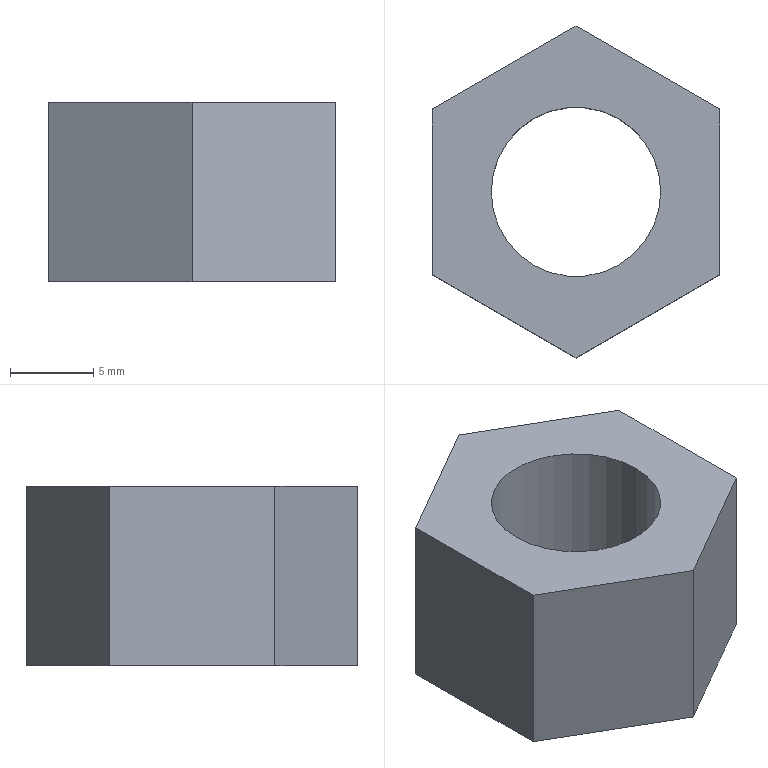Part | SolidWorks | features Extrusion 1, HoleWzd 1, RefAxis 1 | 1 solid | 10 faces | box 17.3 x 19.976 x 10.8 mm | volume 1917 mm3 | plane 8 | cylinder 2 | commonest cylinder face diameters 10.2 x2
STEP:
#1=CARTESIAN_POINT('',(-5.1,0.,-5.4));
#2=VERTEX_POINT('',#1);
#3=CARTESIAN_POINT('',(5.1,0.,-5.4));
#4=VERTEX_POINT('',#3);
#5=CARTESIAN_POINT('',(0.,0.,-5.4));
#6=DIRECTION('',(0.,0.,1.));
#7=DIRECTION('',(1.,0.,0.));
#8=AXIS2_PLACEMENT_3D('',#5,#6,#7);
#9=CIRCLE('',#8,5.1);
#10=EDGE_CURVE('',#2,#4,#9,.T.);
#11=ORIENTED_EDGE('',*,*,#10,.F.);
#12=CARTESIAN_POINT('',(-5.1,0.,5.4));
#13=VERTEX_POINT('',#12);
#14=CARTESIAN_POINT('',(-5.1,0.,5.4));
#15=DIRECTION('',(0.,0.,1.));
#16=VECTOR('',#15,1000.);
#17=LINE('',#14,#16);
#18=EDGE_CURVE('',#2,#13,#17,.T.);
#19=ORIENTED_EDGE('',*,*,#18,.T.);
#20=CARTESIAN_POINT('',(5.1,0.,5.4));
#21=VERTEX_POINT('',#20);
#22=CARTESIAN_POINT('',(0.,0.,5.4));
#23=DIRECTION('',(0.,0.,1.));
#24=DIRECTION('',(1.,0.,0.));
#25=AXIS2_PLACEMENT_3D('',#22,#23,#24);
#26=CIRCLE('',#25,5.1);
#27=EDGE_CURVE('',#13,#21,#26,.T.);
#28=ORIENTED_EDGE('',*,*,#27,.T.);
#29=CARTESIAN_POINT('',(5.1,0.,5.4));
#30=DIRECTION('',(0.,0.,1.));
#31=VECTOR('',#30,1000.);
#32=LINE('',#29,#31);
#33=EDGE_CURVE('',#4,#21,#32,.T.);
#34=ORIENTED_EDGE('',*,*,#33,.F.);
#35=EDGE_LOOP('',(#11,#19,#28,#34));
#36=FACE_OUTER_BOUND('',#35,.T.);
#37=CARTESIAN_POINT('',(0.,0.,5.4));
#38=DIRECTION('',(0.,0.,1.));
#39=DIRECTION('',(1.,0.,0.));
#40=AXIS2_PLACEMENT_3D('',#37,#38,#39);
#41=CYLINDRICAL_SURFACE('',#40,5.1);
#42=ADVANCED_FACE('',(#36),#41,.F.);
#43=CARTESIAN_POINT('',(0.,-9.988,-5.4));
#44=VERTEX_POINT('',#43);
#45=CARTESIAN_POINT('',(8.65,-4.994,-5.4));
#46=VERTEX_POINT('',#45);
#47=CARTESIAN_POINT('',(0.,-9.988,-5.4));
#48=DIRECTION('',(0.866,0.5,0.));
#49=VECTOR('',#48,1000.);
#50=LINE('',#47,#49);
#51=EDGE_CURVE('',#44,#46,#50,.T.);
#52=ORIENTED_EDGE('',*,*,#51,.T.);
#53=CARTESIAN_POINT('',(8.65,-4.994,5.4));
#54=VERTEX_POINT('',#53);
#55=CARTESIAN_POINT('',(8.65,-4.994,5.4));
#56=DIRECTION('',(0.,0.,-1.));
#57=VECTOR('',#56,1000.);
#58=LINE('',#55,#57);
#59=EDGE_CURVE('',#54,#46,#58,.T.);
#60=ORIENTED_EDGE('',*,*,#59,.F.);
#61=CARTESIAN_POINT('',(0.,-9.988,5.4));
#62=VERTEX_POINT('',#61);
#63=CARTESIAN_POINT('',(0.,-9.988,5.4));
#64=DIRECTION('',(0.866,0.5,0.));
#65=VECTOR('',#64,1000.);
#66=LINE('',#63,#65);
#67=EDGE_CURVE('',#62,#54,#66,.T.);
#68=ORIENTED_EDGE('',*,*,#67,.F.);
#69=CARTESIAN_POINT('',(0.,-9.988,5.4));
#70=DIRECTION('',(0.,0.,-1.));
#71=VECTOR('',#70,1000.);
#72=LINE('',#69,#71);
#73=EDGE_CURVE('',#62,#44,#72,.T.);
#74=ORIENTED_EDGE('',*,*,#73,.T.);
#75=EDGE_LOOP('',(#52,#60,#68,#74));
#76=FACE_OUTER_BOUND('',#75,.T.);
#77=CARTESIAN_POINT('',(0.,-9.988,5.4));
#78=DIRECTION('',(-0.5,0.866,0.));
#79=DIRECTION('',(-0.866,-0.5,0.));
#80=AXIS2_PLACEMENT_3D('',#77,#78,#79);
#81=PLANE('',#80);
#82=ADVANCED_FACE('',(#76),#81,.F.);
#83=CARTESIAN_POINT('',(8.65,4.994,-5.4));
#84=VERTEX_POINT('',#83);
#85=CARTESIAN_POINT('',(8.65,-4.994,-5.4));
#86=DIRECTION('',(0.,1.,0.));
#87=VECTOR('',#86,1000.);
#88=LINE('',#85,#87);
#89=EDGE_CURVE('',#46,#84,#88,.T.);
#90=ORIENTED_EDGE('',*,*,#89,.T.);
#91=CARTESIAN_POINT('',(8.65,4.994,5.4));
#92=VERTEX_POINT('',#91);
#93=CARTESIAN_POINT('',(8.65,4.994,5.4));
#94=DIRECTION('',(0.,0.,-1.));
#95=VECTOR('',#94,1000.);
#96=LINE('',#93,#95);
#97=EDGE_CURVE('',#92,#84,#96,.T.);
#98=ORIENTED_EDGE('',*,*,#97,.F.);
#99=CARTESIAN_POINT('',(8.65,-4.994,5.4));
#100=DIRECTION('',(0.,1.,0.));
#101=VECTOR('',#100,1000.);
#102=LINE('',#99,#101);
#103=EDGE_CURVE('',#54,#92,#102,.T.);
#104=ORIENTED_EDGE('',*,*,#103,.F.);
#105=ORIENTED_EDGE('',*,*,#59,.T.);
#106=EDGE_LOOP('',(#90,#98,#104,#105));
#107=FACE_OUTER_BOUND('',#106,.T.);
#108=CARTESIAN_POINT('',(8.65,-4.994,5.4));
#109=DIRECTION('',(-1.,0.,0.));
#110=DIRECTION('',(0.,0.,1.));
#111=AXIS2_PLACEMENT_3D('',#108,#109,#110);
#112=PLANE('',#111);
#113=ADVANCED_FACE('',(#107),#112,.F.);
#114=CARTESIAN_POINT('',(0.,9.988,-5.4));
#115=VERTEX_POINT('',#114);
#116=CARTESIAN_POINT('',(8.65,4.994,-5.4));
#117=DIRECTION('',(-0.866,0.5,0.));
#118=VECTOR('',#117,1000.);
#119=LINE('',#116,#118);
#120=EDGE_CURVE('',#84,#115,#119,.T.);
#121=ORIENTED_EDGE('',*,*,#120,.T.);
#122=CARTESIAN_POINT('',(0.,9.988,5.4));
#123=VERTEX_POINT('',#122);
#124=CARTESIAN_POINT('',(0.,9.988,5.4));
#125=DIRECTION('',(0.,0.,-1.));
#126=VECTOR('',#125,1000.);
#127=LINE('',#124,#126);
#128=EDGE_CURVE('',#123,#115,#127,.T.);
#129=ORIENTED_EDGE('',*,*,#128,.F.);
#130=CARTESIAN_POINT('',(8.65,4.994,5.4));
#131=DIRECTION('',(-0.866,0.5,0.));
#132=VECTOR('',#131,1000.);
#133=LINE('',#130,#132);
#134=EDGE_CURVE('',#92,#123,#133,.T.);
#135=ORIENTED_EDGE('',*,*,#134,.F.);
#136=ORIENTED_EDGE('',*,*,#97,.T.);
#137=EDGE_LOOP('',(#121,#129,#135,#136));
#138=FACE_OUTER_BOUND('',#137,.T.);
#139=CARTESIAN_POINT('',(8.65,4.994,5.4));
#140=DIRECTION('',(-0.5,-0.866,0.));
#141=DIRECTION('',(0.866,-0.5,0.));
#142=AXIS2_PLACEMENT_3D('',#139,#140,#141);
#143=PLANE('',#142);
#144=ADVANCED_FACE('',(#138),#143,.F.);
#145=CARTESIAN_POINT('',(-8.65,4.994,-5.4));
#146=VERTEX_POINT('',#145);
#147=CARTESIAN_POINT('',(0.,9.988,-5.4));
#148=DIRECTION('',(-0.866,-0.5,0.));
#149=VECTOR('',#148,1000.);
#150=LINE('',#147,#149);
#151=EDGE_CURVE('',#115,#146,#150,.T.);
#152=ORIENTED_EDGE('',*,*,#151,.T.);
#153=CARTESIAN_POINT('',(-8.65,4.994,5.4));
#154=VERTEX_POINT('',#153);
#155=CARTESIAN_POINT('',(-8.65,4.994,5.4));
#156=DIRECTION('',(0.,0.,-1.));
#157=VECTOR('',#156,1000.);
#158=LINE('',#155,#157);
#159=EDGE_CURVE('',#154,#146,#158,.T.);
#160=ORIENTED_EDGE('',*,*,#159,.F.);
#161=CARTESIAN_POINT('',(0.,9.988,5.4));
#162=DIRECTION('',(-0.866,-0.5,0.));
#163=VECTOR('',#162,1000.);
#164=LINE('',#161,#163);
#165=EDGE_CURVE('',#123,#154,#164,.T.);
#166=ORIENTED_EDGE('',*,*,#165,.F.);
#167=ORIENTED_EDGE('',*,*,#128,.T.);
#168=EDGE_LOOP('',(#152,#160,#166,#167));
#169=FACE_OUTER_BOUND('',#168,.T.);
#170=CARTESIAN_POINT('',(0.,9.988,5.4));
#171=DIRECTION('',(0.5,-0.866,0.));
#172=DIRECTION('',(0.866,0.5,0.));
#173=AXIS2_PLACEMENT_3D('',#170,#171,#172);
#174=PLANE('',#173);
#175=ADVANCED_FACE('',(#169),#174,.F.);
#176=CARTESIAN_POINT('',(-8.65,-4.994,-5.4));
#177=VERTEX_POINT('',#176);
#178=CARTESIAN_POINT('',(-8.65,4.994,-5.4));
#179=DIRECTION('',(0.,-1.,0.));
#180=VECTOR('',#179,1000.);
#181=LINE('',#178,#180);
#182=EDGE_CURVE('',#146,#177,#181,.T.);
#183=ORIENTED_EDGE('',*,*,#182,.T.);
#184=CARTESIAN_POINT('',(-8.65,-4.994,5.4));
#185=VERTEX_POINT('',#184);
#186=CARTESIAN_POINT('',(-8.65,-4.994,5.4));
#187=DIRECTION('',(0.,0.,-1.));
#188=VECTOR('',#187,1000.);
#189=LINE('',#186,#188);
#190=EDGE_CURVE('',#185,#177,#189,.T.);
#191=ORIENTED_EDGE('',*,*,#190,.F.);
#192=CARTESIAN_POINT('',(-8.65,4.994,5.4));
#193=DIRECTION('',(0.,-1.,0.));
#194=VECTOR('',#193,1000.);
#195=LINE('',#192,#194);
#196=EDGE_CURVE('',#154,#185,#195,.T.);
#197=ORIENTED_EDGE('',*,*,#196,.F.);
#198=ORIENTED_EDGE('',*,*,#159,.T.);
#199=EDGE_LOOP('',(#183,#191,#197,#198));
#200=FACE_OUTER_BOUND('',#199,.T.);
#201=CARTESIAN_POINT('',(-8.65,4.994,5.4));
#202=DIRECTION('',(1.,0.,0.));
#203=DIRECTION('',(0.,0.,-1.));
#204=AXIS2_PLACEMENT_3D('',#201,#202,#203);
#205=PLANE('',#204);
#206=ADVANCED_FACE('',(#200),#205,.F.);
#207=CARTESIAN_POINT('',(-8.65,-4.994,-5.4));
#208=DIRECTION('',(0.866,-0.5,0.));
#209=VECTOR('',#208,1000.);
#210=LINE('',#207,#209);
#211=EDGE_CURVE('',#177,#44,#210,.T.);
#212=ORIENTED_EDGE('',*,*,#211,.T.);
#213=ORIENTED_EDGE('',*,*,#73,.F.);
#214=CARTESIAN_POINT('',(-8.65,-4.994,5.4));
#215=DIRECTION('',(0.866,-0.5,0.));
#216=VECTOR('',#215,1000.);
#217=LINE('',#214,#216);
#218=EDGE_CURVE('',#185,#62,#217,.T.);
#219=ORIENTED_EDGE('',*,*,#218,.F.);
#220=ORIENTED_EDGE('',*,*,#190,.T.);
#221=EDGE_LOOP('',(#212,#213,#219,#220));
#222=FACE_OUTER_BOUND('',#221,.T.);
#223=CARTESIAN_POINT('',(-8.65,-4.994,5.4));
#224=DIRECTION('',(0.5,0.866,0.));
#225=DIRECTION('',(-0.866,0.5,0.));
#226=AXIS2_PLACEMENT_3D('',#223,#224,#225);
#227=PLANE('',#226);
#228=ADVANCED_FACE('',(#222),#227,.F.);
#229=CARTESIAN_POINT('',(0.,0.,5.4));
#230=DIRECTION('',(0.,0.,1.));
#231=DIRECTION('',(1.,0.,0.));
#232=AXIS2_PLACEMENT_3D('',#229,#230,#231);
#233=CIRCLE('',#232,5.1);
#234=EDGE_CURVE('',#21,#13,#233,.T.);
#235=ORIENTED_EDGE('',*,*,#234,.F.);
#236=ORIENTED_EDGE('',*,*,#27,.F.);
#237=EDGE_LOOP('',(#235,#236));
#238=FACE_BOUND('',#237,.T.);
#239=ORIENTED_EDGE('',*,*,#67,.T.);
#240=ORIENTED_EDGE('',*,*,#103,.T.);
#241=ORIENTED_EDGE('',*,*,#134,.T.);
#242=ORIENTED_EDGE('',*,*,#165,.T.);
#243=ORIENTED_EDGE('',*,*,#196,.T.);
#244=ORIENTED_EDGE('',*,*,#218,.T.);
#245=EDGE_LOOP('',(#239,#240,#241,#242,#243,#244));
#246=FACE_OUTER_BOUND('',#245,.T.);
#247=CARTESIAN_POINT('',(0.,0.,5.4));
#248=DIRECTION('',(0.,0.,1.));
#249=DIRECTION('',(1.,0.,0.));
#250=AXIS2_PLACEMENT_3D('',#247,#248,#249);
#251=PLANE('',#250);
#252=ADVANCED_FACE('',(#238,#246),#251,.T.);
#253=CARTESIAN_POINT('',(0.,0.,-5.4));
#254=DIRECTION('',(0.,0.,1.));
#255=DIRECTION('',(1.,0.,0.));
#256=AXIS2_PLACEMENT_3D('',#253,#254,#255);
#257=CIRCLE('',#256,5.1);
#258=EDGE_CURVE('',#4,#2,#257,.T.);
#259=ORIENTED_EDGE('',*,*,#258,.T.);
#260=ORIENTED_EDGE('',*,*,#10,.T.);
#261=EDGE_LOOP('',(#259,#260));
#262=FACE_BOUND('',#261,.T.);
#263=ORIENTED_EDGE('',*,*,#51,.F.);
#264=ORIENTED_EDGE('',*,*,#211,.F.);
#265=ORIENTED_EDGE('',*,*,#182,.F.);
#266=ORIENTED_EDGE('',*,*,#151,.F.);
#267=ORIENTED_EDGE('',*,*,#120,.F.);
#268=ORIENTED_EDGE('',*,*,#89,.F.);
#269=EDGE_LOOP('',(#263,#264,#265,#266,#267,#268));
#270=FACE_OUTER_BOUND('',#269,.T.);
#271=CARTESIAN_POINT('',(0.,0.,-5.4));
#272=DIRECTION('',(0.,0.,1.));
#273=DIRECTION('',(1.,0.,0.));
#274=AXIS2_PLACEMENT_3D('',#271,#272,#273);
#275=PLANE('',#274);
#276=ADVANCED_FACE('',(#262,#270),#275,.F.);
#277=ORIENTED_EDGE('',*,*,#18,.F.);
#278=ORIENTED_EDGE('',*,*,#258,.F.);
#279=ORIENTED_EDGE('',*,*,#33,.T.);
#280=ORIENTED_EDGE('',*,*,#234,.T.);
#281=EDGE_LOOP('',(#277,#278,#279,#280));
#282=FACE_OUTER_BOUND('',#281,.T.);
#283=CARTESIAN_POINT('',(0.,0.,5.4));
#284=DIRECTION('',(0.,0.,1.));
#285=DIRECTION('',(1.,0.,0.));
#286=AXIS2_PLACEMENT_3D('',#283,#284,#285);
#287=CYLINDRICAL_SURFACE('',#286,5.1);
#288=ADVANCED_FACE('',(#282),#287,.F.);
#289=CLOSED_SHELL('',(#42,#82,#113,#144,#175,#206,#228,#252,#276,#288));
#290=MANIFOLD_SOLID_BREP('',#289);
#291=CARTESIAN_POINT('',(0.,0.,0.));
#292=DIRECTION('',(0.,0.,1.));
#293=DIRECTION('',(1.,0.,0.));
#294=AXIS2_PLACEMENT_3D('',#291,#292,#293);
#295=(LENGTH_UNIT()NAMED_UNIT(*)SI_UNIT(.MILLI.,.METRE.));
#296=UNCERTAINTY_MEASURE_WITH_UNIT(LENGTH_MEASURE(0.00001),#295,'','');
#297=(NAMED_UNIT(*)PLANE_ANGLE_UNIT()SI_UNIT($,.RADIAN.));
#298=(NAMED_UNIT(*)SI_UNIT($,.STERADIAN.)SOLID_ANGLE_UNIT());
#299=(GEOMETRIC_REPRESENTATION_CONTEXT(3)GLOBAL_UNCERTAINTY_ASSIGNED_CONTEXT((#296))GLOBAL_UNIT_ASSIGNED_CONTEXT((#295,#297,#298))REPRESENTATION_CONTEXT('',''));
#300=ADVANCED_BREP_SHAPE_REPRESENTATION('',(#290,#294),#299);